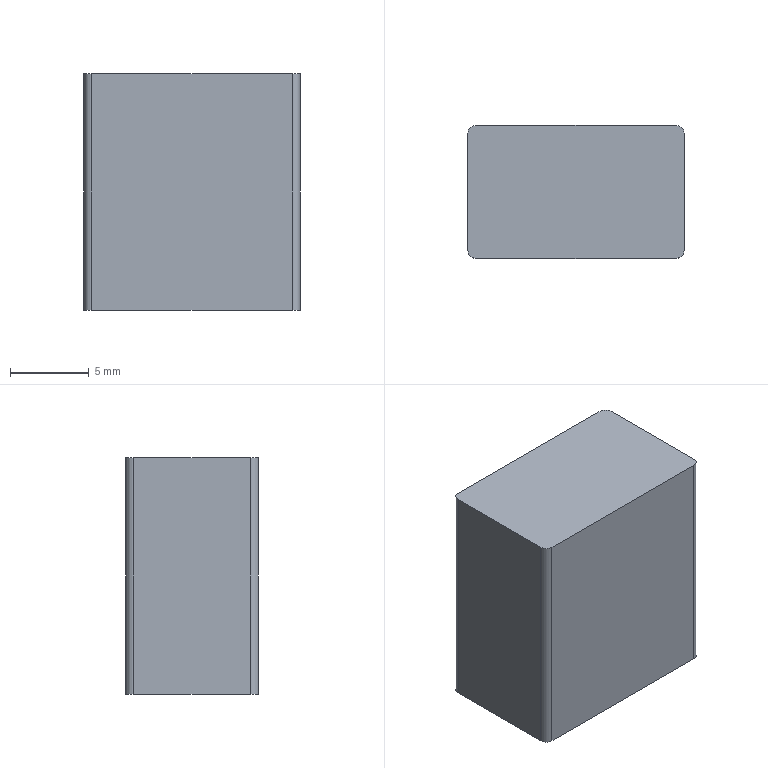Part | NX | features BREP 1 | 1 solid | 10 faces | box 13.7 x 8.4 x 15 mm | volume 1723 mm3 | plane 6 | cylinder 4 | commonest cylinder face diameters 1 x4
STEP:
#1=CARTESIAN_POINT('',(-6.35,4.2,-25.6));
#2=VERTEX_POINT('',#1);
#3=CARTESIAN_POINT('',(-6.85,3.7,-25.6));
#4=VERTEX_POINT('',#3);
#5=CARTESIAN_POINT('',(-6.35,3.7,-25.6));
#6=DIRECTION('',(0.,0.,1.));
#7=DIRECTION('',(1.,0.,0.));
#8=AXIS2_PLACEMENT_3D('',#5,#6,#7);
#9=CIRCLE('',#8,0.5);
#10=EDGE_CURVE('',#2,#4,#9,.T.);
#11=ORIENTED_EDGE('',*,*,#10,.F.);
#12=CARTESIAN_POINT('',(-6.35,4.2,-40.6));
#13=VERTEX_POINT('',#12);
#14=CARTESIAN_POINT('',(-6.35,4.2,-40.6));
#15=DIRECTION('',(0.,0.,1.));
#16=VECTOR('',#15,1000.);
#17=LINE('',#14,#16);
#18=EDGE_CURVE('',#13,#2,#17,.T.);
#19=ORIENTED_EDGE('',*,*,#18,.F.);
#20=CARTESIAN_POINT('',(-6.85,3.7,-40.6));
#21=VERTEX_POINT('',#20);
#22=CARTESIAN_POINT('',(-6.35,3.7,-40.6));
#23=DIRECTION('',(0.,0.,1.));
#24=DIRECTION('',(1.,0.,0.));
#25=AXIS2_PLACEMENT_3D('',#22,#23,#24);
#26=CIRCLE('',#25,0.5);
#27=EDGE_CURVE('',#13,#21,#26,.T.);
#28=ORIENTED_EDGE('',*,*,#27,.T.);
#29=CARTESIAN_POINT('',(-6.85,3.7,-40.6));
#30=DIRECTION('',(0.,0.,1.));
#31=VECTOR('',#30,1000.);
#32=LINE('',#29,#31);
#33=EDGE_CURVE('',#21,#4,#32,.T.);
#34=ORIENTED_EDGE('',*,*,#33,.T.);
#35=EDGE_LOOP('',(#11,#19,#28,#34));
#36=FACE_BOUND('',#35,.T.);
#37=CARTESIAN_POINT('',(-6.35,3.7,-40.6));
#38=DIRECTION('',(0.,0.,1.));
#39=DIRECTION('',(-1.,0.,0.));
#40=AXIS2_PLACEMENT_3D('',#37,#38,#39);
#41=CYLINDRICAL_SURFACE('',#40,0.5);
#42=ADVANCED_FACE('',(#36),#41,.T.);
#43=CARTESIAN_POINT('',(-6.85,-3.7,-25.6));
#44=VERTEX_POINT('',#43);
#45=CARTESIAN_POINT('',(-6.85,-3.7,-25.6));
#46=DIRECTION('',(0.,1.,0.));
#47=VECTOR('',#46,1000.);
#48=LINE('',#45,#47);
#49=EDGE_CURVE('',#44,#4,#48,.T.);
#50=ORIENTED_EDGE('',*,*,#49,.T.);
#51=ORIENTED_EDGE('',*,*,#33,.F.);
#52=CARTESIAN_POINT('',(-6.85,-3.7,-40.6));
#53=VERTEX_POINT('',#52);
#54=CARTESIAN_POINT('',(-6.85,-3.7,-40.6));
#55=DIRECTION('',(0.,1.,0.));
#56=VECTOR('',#55,1000.);
#57=LINE('',#54,#56);
#58=EDGE_CURVE('',#53,#21,#57,.T.);
#59=ORIENTED_EDGE('',*,*,#58,.F.);
#60=CARTESIAN_POINT('',(-6.85,-3.7,-40.6));
#61=DIRECTION('',(0.,0.,1.));
#62=VECTOR('',#61,1000.);
#63=LINE('',#60,#62);
#64=EDGE_CURVE('',#53,#44,#63,.T.);
#65=ORIENTED_EDGE('',*,*,#64,.T.);
#66=EDGE_LOOP('',(#50,#51,#59,#65));
#67=FACE_BOUND('',#66,.T.);
#68=CARTESIAN_POINT('',(-6.85,-3.7,-40.6));
#69=DIRECTION('',(1.,0.,0.));
#70=DIRECTION('',(0.,0.,1.));
#71=AXIS2_PLACEMENT_3D('',#68,#69,#70);
#72=PLANE('',#71);
#73=ADVANCED_FACE('',(#67),#72,.F.);
#74=CARTESIAN_POINT('',(-6.35,-4.2,-25.6));
#75=VERTEX_POINT('',#74);
#76=CARTESIAN_POINT('',(-6.35,-3.7,-25.6));
#77=DIRECTION('',(0.,0.,1.));
#78=DIRECTION('',(1.,0.,0.));
#79=AXIS2_PLACEMENT_3D('',#76,#77,#78);
#80=CIRCLE('',#79,0.5);
#81=EDGE_CURVE('',#44,#75,#80,.T.);
#82=ORIENTED_EDGE('',*,*,#81,.F.);
#83=ORIENTED_EDGE('',*,*,#64,.F.);
#84=CARTESIAN_POINT('',(-6.35,-4.2,-40.6));
#85=VERTEX_POINT('',#84);
#86=CARTESIAN_POINT('',(-6.35,-3.7,-40.6));
#87=DIRECTION('',(0.,0.,1.));
#88=DIRECTION('',(1.,0.,0.));
#89=AXIS2_PLACEMENT_3D('',#86,#87,#88);
#90=CIRCLE('',#89,0.5);
#91=EDGE_CURVE('',#53,#85,#90,.T.);
#92=ORIENTED_EDGE('',*,*,#91,.T.);
#93=CARTESIAN_POINT('',(-6.35,-4.2,-40.6));
#94=DIRECTION('',(0.,0.,1.));
#95=VECTOR('',#94,1000.);
#96=LINE('',#93,#95);
#97=EDGE_CURVE('',#85,#75,#96,.T.);
#98=ORIENTED_EDGE('',*,*,#97,.T.);
#99=EDGE_LOOP('',(#82,#83,#92,#98));
#100=FACE_BOUND('',#99,.T.);
#101=CARTESIAN_POINT('',(-6.35,-3.7,-40.6));
#102=DIRECTION('',(0.,0.,1.));
#103=DIRECTION('',(-1.,0.,0.));
#104=AXIS2_PLACEMENT_3D('',#101,#102,#103);
#105=CYLINDRICAL_SURFACE('',#104,0.5);
#106=ADVANCED_FACE('',(#100),#105,.T.);
#107=CARTESIAN_POINT('',(6.35,-4.2,-25.6));
#108=VERTEX_POINT('',#107);
#109=CARTESIAN_POINT('',(6.35,-4.2,-25.6));
#110=DIRECTION('',(-1.,0.,0.));
#111=VECTOR('',#110,1000.);
#112=LINE('',#109,#111);
#113=EDGE_CURVE('',#108,#75,#112,.T.);
#114=ORIENTED_EDGE('',*,*,#113,.T.);
#115=ORIENTED_EDGE('',*,*,#97,.F.);
#116=CARTESIAN_POINT('',(6.35,-4.2,-40.6));
#117=VERTEX_POINT('',#116);
#118=CARTESIAN_POINT('',(6.35,-4.2,-40.6));
#119=DIRECTION('',(-1.,0.,0.));
#120=VECTOR('',#119,1000.);
#121=LINE('',#118,#120);
#122=EDGE_CURVE('',#117,#85,#121,.T.);
#123=ORIENTED_EDGE('',*,*,#122,.F.);
#124=CARTESIAN_POINT('',(6.35,-4.2,-40.6));
#125=DIRECTION('',(0.,0.,1.));
#126=VECTOR('',#125,1000.);
#127=LINE('',#124,#126);
#128=EDGE_CURVE('',#117,#108,#127,.T.);
#129=ORIENTED_EDGE('',*,*,#128,.T.);
#130=EDGE_LOOP('',(#114,#115,#123,#129));
#131=FACE_BOUND('',#130,.T.);
#132=CARTESIAN_POINT('',(6.35,-4.2,-40.6));
#133=DIRECTION('',(0.,1.,0.));
#134=DIRECTION('',(1.,0.,0.));
#135=AXIS2_PLACEMENT_3D('',#132,#133,#134);
#136=PLANE('',#135);
#137=ADVANCED_FACE('',(#131),#136,.F.);
#138=CARTESIAN_POINT('',(6.85,-3.7,-25.6));
#139=VERTEX_POINT('',#138);
#140=CARTESIAN_POINT('',(6.35,-3.7,-25.6));
#141=DIRECTION('',(0.,0.,1.));
#142=DIRECTION('',(1.,0.,0.));
#143=AXIS2_PLACEMENT_3D('',#140,#141,#142);
#144=CIRCLE('',#143,0.5);
#145=EDGE_CURVE('',#108,#139,#144,.T.);
#146=ORIENTED_EDGE('',*,*,#145,.F.);
#147=ORIENTED_EDGE('',*,*,#128,.F.);
#148=CARTESIAN_POINT('',(6.85,-3.7,-40.6));
#149=VERTEX_POINT('',#148);
#150=CARTESIAN_POINT('',(6.35,-3.7,-40.6));
#151=DIRECTION('',(0.,0.,1.));
#152=DIRECTION('',(1.,0.,0.));
#153=AXIS2_PLACEMENT_3D('',#150,#151,#152);
#154=CIRCLE('',#153,0.5);
#155=EDGE_CURVE('',#117,#149,#154,.T.);
#156=ORIENTED_EDGE('',*,*,#155,.T.);
#157=CARTESIAN_POINT('',(6.85,-3.7,-40.6));
#158=DIRECTION('',(0.,0.,1.));
#159=VECTOR('',#158,1000.);
#160=LINE('',#157,#159);
#161=EDGE_CURVE('',#149,#139,#160,.T.);
#162=ORIENTED_EDGE('',*,*,#161,.T.);
#163=EDGE_LOOP('',(#146,#147,#156,#162));
#164=FACE_BOUND('',#163,.T.);
#165=CARTESIAN_POINT('',(6.35,-3.7,-40.6));
#166=DIRECTION('',(0.,0.,1.));
#167=DIRECTION('',(-1.,0.,0.));
#168=AXIS2_PLACEMENT_3D('',#165,#166,#167);
#169=CYLINDRICAL_SURFACE('',#168,0.5);
#170=ADVANCED_FACE('',(#164),#169,.T.);
#171=CARTESIAN_POINT('',(6.85,3.7,-25.6));
#172=VERTEX_POINT('',#171);
#173=CARTESIAN_POINT('',(6.85,3.7,-25.6));
#174=DIRECTION('',(0.,-1.,0.));
#175=VECTOR('',#174,1000.);
#176=LINE('',#173,#175);
#177=EDGE_CURVE('',#172,#139,#176,.T.);
#178=ORIENTED_EDGE('',*,*,#177,.T.);
#179=ORIENTED_EDGE('',*,*,#161,.F.);
#180=CARTESIAN_POINT('',(6.85,3.7,-40.6));
#181=VERTEX_POINT('',#180);
#182=CARTESIAN_POINT('',(6.85,3.7,-40.6));
#183=DIRECTION('',(0.,-1.,0.));
#184=VECTOR('',#183,1000.);
#185=LINE('',#182,#184);
#186=EDGE_CURVE('',#181,#149,#185,.T.);
#187=ORIENTED_EDGE('',*,*,#186,.F.);
#188=CARTESIAN_POINT('',(6.85,3.7,-40.6));
#189=DIRECTION('',(0.,0.,1.));
#190=VECTOR('',#189,1000.);
#191=LINE('',#188,#190);
#192=EDGE_CURVE('',#181,#172,#191,.T.);
#193=ORIENTED_EDGE('',*,*,#192,.T.);
#194=EDGE_LOOP('',(#178,#179,#187,#193));
#195=FACE_BOUND('',#194,.T.);
#196=CARTESIAN_POINT('',(6.85,3.7,-40.6));
#197=DIRECTION('',(-1.,0.,0.));
#198=DIRECTION('',(0.,0.,-1.));
#199=AXIS2_PLACEMENT_3D('',#196,#197,#198);
#200=PLANE('',#199);
#201=ADVANCED_FACE('',(#195),#200,.F.);
#202=CARTESIAN_POINT('',(6.35,4.2,-25.6));
#203=VERTEX_POINT('',#202);
#204=CARTESIAN_POINT('',(6.35,3.7,-25.6));
#205=DIRECTION('',(0.,0.,1.));
#206=DIRECTION('',(1.,0.,0.));
#207=AXIS2_PLACEMENT_3D('',#204,#205,#206);
#208=CIRCLE('',#207,0.5);
#209=EDGE_CURVE('',#172,#203,#208,.T.);
#210=ORIENTED_EDGE('',*,*,#209,.F.);
#211=ORIENTED_EDGE('',*,*,#192,.F.);
#212=CARTESIAN_POINT('',(6.35,4.2,-40.6));
#213=VERTEX_POINT('',#212);
#214=CARTESIAN_POINT('',(6.35,3.7,-40.6));
#215=DIRECTION('',(0.,0.,1.));
#216=DIRECTION('',(1.,0.,0.));
#217=AXIS2_PLACEMENT_3D('',#214,#215,#216);
#218=CIRCLE('',#217,0.5);
#219=EDGE_CURVE('',#181,#213,#218,.T.);
#220=ORIENTED_EDGE('',*,*,#219,.T.);
#221=CARTESIAN_POINT('',(6.35,4.2,-40.6));
#222=DIRECTION('',(0.,0.,1.));
#223=VECTOR('',#222,1000.);
#224=LINE('',#221,#223);
#225=EDGE_CURVE('',#213,#203,#224,.T.);
#226=ORIENTED_EDGE('',*,*,#225,.T.);
#227=EDGE_LOOP('',(#210,#211,#220,#226));
#228=FACE_BOUND('',#227,.T.);
#229=CARTESIAN_POINT('',(6.35,3.7,-40.6));
#230=DIRECTION('',(0.,0.,1.));
#231=DIRECTION('',(-1.,0.,0.));
#232=AXIS2_PLACEMENT_3D('',#229,#230,#231);
#233=CYLINDRICAL_SURFACE('',#232,0.5);
#234=ADVANCED_FACE('',(#228),#233,.T.);
#235=CARTESIAN_POINT('',(-6.35,4.2,-25.6));
#236=DIRECTION('',(1.,0.,0.));
#237=VECTOR('',#236,1000.);
#238=LINE('',#235,#237);
#239=EDGE_CURVE('',#2,#203,#238,.T.);
#240=ORIENTED_EDGE('',*,*,#239,.T.);
#241=ORIENTED_EDGE('',*,*,#225,.F.);
#242=CARTESIAN_POINT('',(-6.35,4.2,-40.6));
#243=DIRECTION('',(1.,0.,0.));
#244=VECTOR('',#243,1000.);
#245=LINE('',#242,#244);
#246=EDGE_CURVE('',#13,#213,#245,.T.);
#247=ORIENTED_EDGE('',*,*,#246,.F.);
#248=ORIENTED_EDGE('',*,*,#18,.T.);
#249=EDGE_LOOP('',(#240,#241,#247,#248));
#250=FACE_BOUND('',#249,.T.);
#251=CARTESIAN_POINT('',(-6.35,4.2,-40.6));
#252=DIRECTION('',(0.,-1.,0.));
#253=DIRECTION('',(0.,0.,1.));
#254=AXIS2_PLACEMENT_3D('',#251,#252,#253);
#255=PLANE('',#254);
#256=ADVANCED_FACE('',(#250),#255,.F.);
#257=ORIENTED_EDGE('',*,*,#27,.F.);
#258=ORIENTED_EDGE('',*,*,#246,.T.);
#259=ORIENTED_EDGE('',*,*,#219,.F.);
#260=ORIENTED_EDGE('',*,*,#186,.T.);
#261=ORIENTED_EDGE('',*,*,#155,.F.);
#262=ORIENTED_EDGE('',*,*,#122,.T.);
#263=ORIENTED_EDGE('',*,*,#91,.F.);
#264=ORIENTED_EDGE('',*,*,#58,.T.);
#265=EDGE_LOOP('',(#257,#258,#259,#260,#261,#262,#263,#264));
#266=FACE_BOUND('',#265,.T.);
#267=CARTESIAN_POINT('',(-6.35,3.7,-40.6));
#268=DIRECTION('',(0.,0.,1.));
#269=DIRECTION('',(-1.,0.,0.));
#270=AXIS2_PLACEMENT_3D('',#267,#268,#269);
#271=PLANE('',#270);
#272=ADVANCED_FACE('',(#266),#271,.F.);
#273=ORIENTED_EDGE('',*,*,#10,.T.);
#274=ORIENTED_EDGE('',*,*,#49,.F.);
#275=ORIENTED_EDGE('',*,*,#81,.T.);
#276=ORIENTED_EDGE('',*,*,#113,.F.);
#277=ORIENTED_EDGE('',*,*,#145,.T.);
#278=ORIENTED_EDGE('',*,*,#177,.F.);
#279=ORIENTED_EDGE('',*,*,#209,.T.);
#280=ORIENTED_EDGE('',*,*,#239,.F.);
#281=EDGE_LOOP('',(#273,#274,#275,#276,#277,#278,#279,#280));
#282=FACE_BOUND('',#281,.T.);
#283=CARTESIAN_POINT('',(-6.35,3.7,-25.6));
#284=DIRECTION('',(0.,0.,1.));
#285=DIRECTION('',(-1.,0.,0.));
#286=AXIS2_PLACEMENT_3D('',#283,#284,#285);
#287=PLANE('',#286);
#288=ADVANCED_FACE('',(#282),#287,.T.);
#289=CLOSED_SHELL('',(#42,#73,#106,#137,#170,#201,#234,#256,#272,#288));
#290=MANIFOLD_SOLID_BREP('',#289);
#291=(LENGTH_UNIT()NAMED_UNIT(*)SI_UNIT(.MILLI.,.METRE.));
#292=UNCERTAINTY_MEASURE_WITH_UNIT(LENGTH_MEASURE(0.00001),#291,'','');
#293=(NAMED_UNIT(*)PLANE_ANGLE_UNIT()SI_UNIT($,.RADIAN.));
#294=(NAMED_UNIT(*)SI_UNIT($,.STERADIAN.)SOLID_ANGLE_UNIT());
#295=(GEOMETRIC_REPRESENTATION_CONTEXT(3)GLOBAL_UNCERTAINTY_ASSIGNED_CONTEXT((#292))GLOBAL_UNIT_ASSIGNED_CONTEXT((#291,#293,#294))REPRESENTATION_CONTEXT('',''));
#296=ADVANCED_BREP_SHAPE_REPRESENTATION('',(#290),#295);